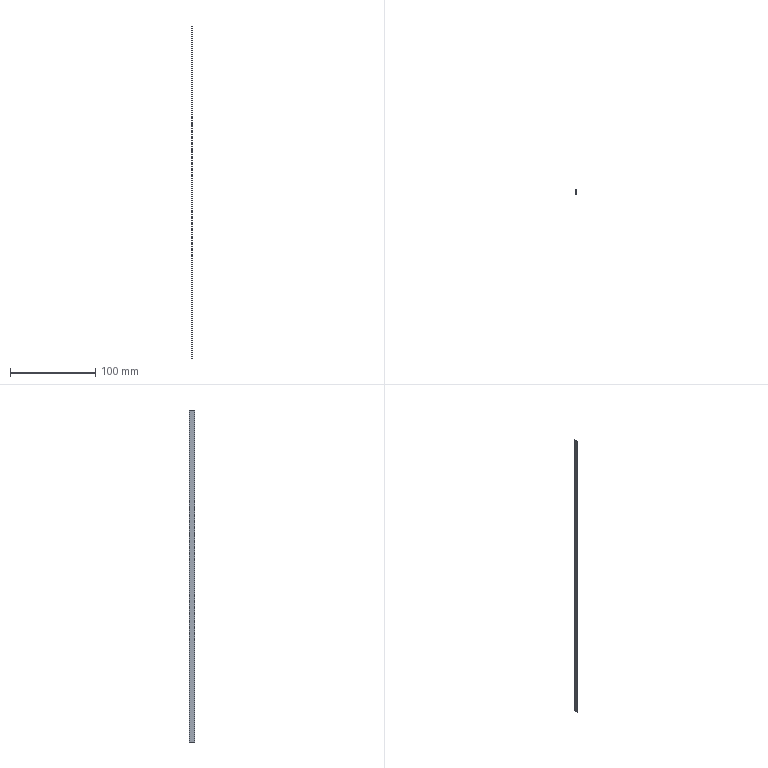Part | NX | features BREP 1 | 1 solid | 6 faces | box 0.3 x 6 x 390 mm | volume 702 mm3 | plane 6
STEP:
#1=CARTESIAN_POINT('',(0.15,6.,-250.));
#2=VERTEX_POINT('',#1);
#3=CARTESIAN_POINT('',(-0.15,6.,-250.));
#4=VERTEX_POINT('',#3);
#5=CARTESIAN_POINT('',(-0.15,6.,-250.));
#6=DIRECTION('',(-1.,0.,0.));
#7=VECTOR('',#6,1000.);
#8=LINE('',#5,#7);
#9=EDGE_CURVE('',#2,#4,#8,.T.);
#10=ORIENTED_EDGE('',*,*,#9,.F.);
#11=CARTESIAN_POINT('',(0.15,0.,-250.));
#12=VERTEX_POINT('',#11);
#13=CARTESIAN_POINT('',(0.15,6.,-250.));
#14=DIRECTION('',(0.,1.,0.));
#15=VECTOR('',#14,1000.);
#16=LINE('',#13,#15);
#17=EDGE_CURVE('',#12,#2,#16,.T.);
#18=ORIENTED_EDGE('',*,*,#17,.F.);
#19=CARTESIAN_POINT('',(-0.15,0.,-250.));
#20=VERTEX_POINT('',#19);
#21=CARTESIAN_POINT('',(0.15,0.,-250.));
#22=DIRECTION('',(1.,0.,0.));
#23=VECTOR('',#22,1000.);
#24=LINE('',#21,#23);
#25=EDGE_CURVE('',#20,#12,#24,.T.);
#26=ORIENTED_EDGE('',*,*,#25,.F.);
#27=CARTESIAN_POINT('',(-0.15,0.,-250.));
#28=DIRECTION('',(0.,-1.,0.));
#29=VECTOR('',#28,1000.);
#30=LINE('',#27,#29);
#31=EDGE_CURVE('',#4,#20,#30,.T.);
#32=ORIENTED_EDGE('',*,*,#31,.F.);
#33=EDGE_LOOP('',(#10,#18,#26,#32));
#34=FACE_BOUND('',#33,.T.);
#35=CARTESIAN_POINT('',(0.,0.,-250.));
#36=DIRECTION('',(0.,0.,1.));
#37=DIRECTION('',(1.,0.,0.));
#38=AXIS2_PLACEMENT_3D('',#35,#36,#37);
#39=PLANE('',#38);
#40=ADVANCED_FACE('',(#34),#39,.F.);
#41=CARTESIAN_POINT('',(0.15,0.,140.));
#42=VERTEX_POINT('',#41);
#43=CARTESIAN_POINT('',(0.15,0.,-140.));
#44=DIRECTION('',(0.,0.,1.));
#45=VECTOR('',#44,1000.);
#46=LINE('',#43,#45);
#47=EDGE_CURVE('',#12,#42,#46,.T.);
#48=ORIENTED_EDGE('',*,*,#47,.F.);
#49=ORIENTED_EDGE('',*,*,#17,.T.);
#50=CARTESIAN_POINT('',(0.15,6.,140.));
#51=VERTEX_POINT('',#50);
#52=CARTESIAN_POINT('',(0.15,6.,-140.));
#53=DIRECTION('',(0.,0.,-1.));
#54=VECTOR('',#53,1000.);
#55=LINE('',#52,#54);
#56=EDGE_CURVE('',#51,#2,#55,.T.);
#57=ORIENTED_EDGE('',*,*,#56,.F.);
#58=CARTESIAN_POINT('',(0.15,0.,140.));
#59=DIRECTION('',(0.,1.,0.));
#60=VECTOR('',#59,1000.);
#61=LINE('',#58,#60);
#62=EDGE_CURVE('',#42,#51,#61,.T.);
#63=ORIENTED_EDGE('',*,*,#62,.F.);
#64=EDGE_LOOP('',(#48,#49,#57,#63));
#65=FACE_BOUND('',#64,.T.);
#66=CARTESIAN_POINT('',(0.15,0.,-140.));
#67=DIRECTION('',(1.,0.,0.));
#68=DIRECTION('',(0.,0.,-1.));
#69=AXIS2_PLACEMENT_3D('',#66,#67,#68);
#70=PLANE('',#69);
#71=ADVANCED_FACE('',(#65),#70,.T.);
#72=CARTESIAN_POINT('',(-0.15,0.,140.));
#73=VERTEX_POINT('',#72);
#74=CARTESIAN_POINT('',(-0.15,0.,-140.));
#75=DIRECTION('',(0.,0.,1.));
#76=VECTOR('',#75,1000.);
#77=LINE('',#74,#76);
#78=EDGE_CURVE('',#20,#73,#77,.T.);
#79=ORIENTED_EDGE('',*,*,#78,.F.);
#80=ORIENTED_EDGE('',*,*,#25,.T.);
#81=ORIENTED_EDGE('',*,*,#47,.T.);
#82=CARTESIAN_POINT('',(0.,0.,140.));
#83=DIRECTION('',(1.,0.,0.));
#84=VECTOR('',#83,1000.);
#85=LINE('',#82,#84);
#86=EDGE_CURVE('',#73,#42,#85,.T.);
#87=ORIENTED_EDGE('',*,*,#86,.F.);
#88=EDGE_LOOP('',(#79,#80,#81,#87));
#89=FACE_BOUND('',#88,.T.);
#90=CARTESIAN_POINT('',(-0.15,0.,-140.));
#91=DIRECTION('',(0.,-1.,0.));
#92=DIRECTION('',(0.,0.,-1.));
#93=AXIS2_PLACEMENT_3D('',#90,#91,#92);
#94=PLANE('',#93);
#95=ADVANCED_FACE('',(#89),#94,.T.);
#96=CARTESIAN_POINT('',(-0.15,6.,140.));
#97=VERTEX_POINT('',#96);
#98=CARTESIAN_POINT('',(-0.15,6.,140.));
#99=DIRECTION('',(0.,1.,0.));
#100=VECTOR('',#99,1000.);
#101=LINE('',#98,#100);
#102=EDGE_CURVE('',#73,#97,#101,.T.);
#103=ORIENTED_EDGE('',*,*,#102,.F.);
#104=ORIENTED_EDGE('',*,*,#86,.T.);
#105=ORIENTED_EDGE('',*,*,#62,.T.);
#106=CARTESIAN_POINT('',(0.15,6.,140.));
#107=DIRECTION('',(1.,0.,0.));
#108=VECTOR('',#107,1000.);
#109=LINE('',#106,#108);
#110=EDGE_CURVE('',#97,#51,#109,.T.);
#111=ORIENTED_EDGE('',*,*,#110,.F.);
#112=EDGE_LOOP('',(#103,#104,#105,#111));
#113=FACE_BOUND('',#112,.T.);
#114=CARTESIAN_POINT('',(0.,0.,140.));
#115=DIRECTION('',(0.,0.,1.));
#116=DIRECTION('',(1.,0.,0.));
#117=AXIS2_PLACEMENT_3D('',#114,#115,#116);
#118=PLANE('',#117);
#119=ADVANCED_FACE('',(#113),#118,.T.);
#120=ORIENTED_EDGE('',*,*,#56,.T.);
#121=ORIENTED_EDGE('',*,*,#9,.T.);
#122=CARTESIAN_POINT('',(-0.15,6.,-140.));
#123=DIRECTION('',(0.,0.,-1.));
#124=VECTOR('',#123,1000.);
#125=LINE('',#122,#124);
#126=EDGE_CURVE('',#97,#4,#125,.T.);
#127=ORIENTED_EDGE('',*,*,#126,.F.);
#128=ORIENTED_EDGE('',*,*,#110,.T.);
#129=EDGE_LOOP('',(#120,#121,#127,#128));
#130=FACE_BOUND('',#129,.T.);
#131=CARTESIAN_POINT('',(0.15,6.,-140.));
#132=DIRECTION('',(0.,1.,0.));
#133=DIRECTION('',(0.,0.,1.));
#134=AXIS2_PLACEMENT_3D('',#131,#132,#133);
#135=PLANE('',#134);
#136=ADVANCED_FACE('',(#130),#135,.T.);
#137=ORIENTED_EDGE('',*,*,#126,.T.);
#138=ORIENTED_EDGE('',*,*,#31,.T.);
#139=ORIENTED_EDGE('',*,*,#78,.T.);
#140=ORIENTED_EDGE('',*,*,#102,.T.);
#141=EDGE_LOOP('',(#137,#138,#139,#140));
#142=FACE_BOUND('',#141,.T.);
#143=CARTESIAN_POINT('',(-0.15,6.,-140.));
#144=DIRECTION('',(-1.,0.,0.));
#145=DIRECTION('',(0.,0.,1.));
#146=AXIS2_PLACEMENT_3D('',#143,#144,#145);
#147=PLANE('',#146);
#148=ADVANCED_FACE('',(#142),#147,.T.);
#149=CLOSED_SHELL('',(#40,#71,#95,#119,#136,#148));
#150=MANIFOLD_SOLID_BREP('',#149);
#151=(LENGTH_UNIT()NAMED_UNIT(*)SI_UNIT(.MILLI.,.METRE.));
#152=UNCERTAINTY_MEASURE_WITH_UNIT(LENGTH_MEASURE(0.00001),#151,'','');
#153=(NAMED_UNIT(*)PLANE_ANGLE_UNIT()SI_UNIT($,.RADIAN.));
#154=(NAMED_UNIT(*)SI_UNIT($,.STERADIAN.)SOLID_ANGLE_UNIT());
#155=(GEOMETRIC_REPRESENTATION_CONTEXT(3)GLOBAL_UNCERTAINTY_ASSIGNED_CONTEXT((#152))GLOBAL_UNIT_ASSIGNED_CONTEXT((#151,#153,#154))REPRESENTATION_CONTEXT('',''));
#156=ADVANCED_BREP_SHAPE_REPRESENTATION('',(#150),#155);